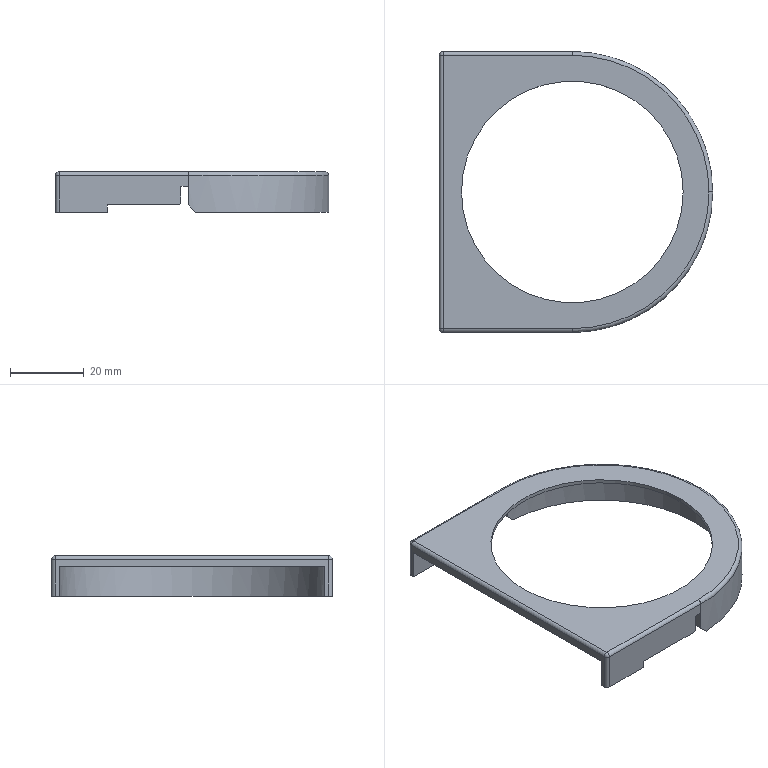Part | SolidWorks | features ICE 8, Fillet 2, Chamfer 1, Stock 1, SurfCut 1 | 1 solid | 39 faces | box 74 x 76 x 11 mm | volume 5943 mm3 | plane 24 | cylinder 11 | torus 2 | sphere 2 | commonest cylinder face diameters 2 x7 60 x2 72 x1 76 x1
STEP:
#1=CARTESIAN_POINT('',(133.,0.,24.));
#2=VERTEX_POINT('',#1);
#3=CARTESIAN_POINT('',(95.,-38.,24.));
#4=VERTEX_POINT('',#3);
#5=CARTESIAN_POINT('',(95.,0.,24.));
#6=DIRECTION('',(0.,0.,-1.));
#7=DIRECTION('',(1.,0.,0.));
#8=AXIS2_PLACEMENT_3D('',#5,#6,#7);
#9=CIRCLE('',#8,38.);
#10=EDGE_CURVE('',#2,#4,#9,.T.);
#11=ORIENTED_EDGE('',*,*,#10,.F.);
#12=CARTESIAN_POINT('',(132.,0.,25.));
#13=VERTEX_POINT('',#12);
#14=CARTESIAN_POINT('',(132.,0.,24.));
#15=DIRECTION('',(0.,-1.,0.));
#16=DIRECTION('',(0.,0.,-1.));
#17=AXIS2_PLACEMENT_3D('',#14,#15,#16);
#18=CIRCLE('',#17,1.);
#19=EDGE_CURVE('',#2,#13,#18,.T.);
#20=ORIENTED_EDGE('',*,*,#19,.T.);
#21=CARTESIAN_POINT('',(95.,-37.,25.));
#22=VERTEX_POINT('',#21);
#23=CARTESIAN_POINT('',(95.,0.,25.));
#24=DIRECTION('',(0.,0.,1.));
#25=DIRECTION('',(1.,0.,0.));
#26=AXIS2_PLACEMENT_3D('',#23,#24,#25);
#27=CIRCLE('',#26,37.);
#28=EDGE_CURVE('',#22,#13,#27,.T.);
#29=ORIENTED_EDGE('',*,*,#28,.F.);
#30=CARTESIAN_POINT('',(95.,-37.,24.));
#31=DIRECTION('',(1.,0.,0.));
#32=DIRECTION('',(0.,0.,-1.));
#33=AXIS2_PLACEMENT_3D('',#30,#31,#32);
#34=CIRCLE('',#33,1.);
#35=EDGE_CURVE('',#22,#4,#34,.T.);
#36=ORIENTED_EDGE('',*,*,#35,.T.);
#37=EDGE_LOOP('',(#11,#20,#29,#36));
#38=FACE_OUTER_BOUND('',#37,.T.);
#39=CARTESIAN_POINT('',(95.,0.,24.));
#40=DIRECTION('',(0.,0.,1.));
#41=DIRECTION('',(1.,0.,0.));
#42=AXIS2_PLACEMENT_3D('',#39,#40,#41);
#43=TOROIDAL_SURFACE('',#42,37.,1.);
#44=ADVANCED_FACE('',(#38),#43,.T.);
#45=CARTESIAN_POINT('',(65.,0.,24.));
#46=VERTEX_POINT('',#45);
#47=CARTESIAN_POINT('',(125.,0.,24.));
#48=VERTEX_POINT('',#47);
#49=CARTESIAN_POINT('',(95.,0.,24.));
#50=DIRECTION('',(0.,0.,1.));
#51=DIRECTION('',(1.,0.,0.));
#52=AXIS2_PLACEMENT_3D('',#49,#50,#51);
#53=CIRCLE('',#52,30.);
#54=EDGE_CURVE('',#46,#48,#53,.T.);
#55=ORIENTED_EDGE('',*,*,#54,.F.);
#56=CARTESIAN_POINT('',(65.,0.,25.));
#57=VERTEX_POINT('',#56);
#58=CARTESIAN_POINT('',(65.,0.,18.));
#59=DIRECTION('',(0.,0.,1.));
#60=VECTOR('',#59,1000.);
#61=LINE('',#58,#60);
#62=EDGE_CURVE('',#46,#57,#61,.T.);
#63=ORIENTED_EDGE('',*,*,#62,.T.);
#64=CARTESIAN_POINT('',(125.,0.,25.));
#65=VERTEX_POINT('',#64);
#66=CARTESIAN_POINT('',(95.,0.,25.));
#67=DIRECTION('',(0.,0.,1.));
#68=DIRECTION('',(1.,0.,0.));
#69=AXIS2_PLACEMENT_3D('',#66,#67,#68);
#70=CIRCLE('',#69,30.);
#71=EDGE_CURVE('',#57,#65,#70,.T.);
#72=ORIENTED_EDGE('',*,*,#71,.T.);
#73=CARTESIAN_POINT('',(125.,0.,18.));
#74=DIRECTION('',(0.,0.,1.));
#75=VECTOR('',#74,1000.);
#76=LINE('',#73,#75);
#77=EDGE_CURVE('',#48,#65,#76,.T.);
#78=ORIENTED_EDGE('',*,*,#77,.F.);
#79=EDGE_LOOP('',(#55,#63,#72,#78));
#80=FACE_OUTER_BOUND('',#79,.T.);
#81=CARTESIAN_POINT('',(95.,0.,18.));
#82=DIRECTION('',(0.,0.,1.));
#83=DIRECTION('',(1.,0.,0.));
#84=AXIS2_PLACEMENT_3D('',#81,#82,#83);
#85=CYLINDRICAL_SURFACE('',#84,30.);
#86=ADVANCED_FACE('',(#80),#85,.F.);
#87=CARTESIAN_POINT('',(95.,0.,24.));
#88=DIRECTION('',(0.,0.,1.));
#89=DIRECTION('',(1.,0.,0.));
#90=AXIS2_PLACEMENT_3D('',#87,#88,#89);
#91=CIRCLE('',#90,30.);
#92=EDGE_CURVE('',#48,#46,#91,.T.);
#93=ORIENTED_EDGE('',*,*,#92,.T.);
#94=ORIENTED_EDGE('',*,*,#54,.T.);
#95=EDGE_LOOP('',(#93,#94));
#96=FACE_BOUND('',#95,.T.);
#97=CARTESIAN_POINT('',(61.,36.,24.));
#98=VERTEX_POINT('',#97);
#99=CARTESIAN_POINT('',(61.,-36.,24.));
#100=VERTEX_POINT('',#99);
#101=CARTESIAN_POINT('',(61.,-34.,24.));
#102=DIRECTION('',(0.,-1.,0.));
#103=VECTOR('',#102,1000.);
#104=LINE('',#101,#103);
#105=EDGE_CURVE('',#98,#100,#104,.T.);
#106=ORIENTED_EDGE('',*,*,#105,.F.);
#107=CARTESIAN_POINT('',(95.,36.,24.));
#108=VERTEX_POINT('',#107);
#109=CARTESIAN_POINT('',(61.,36.,24.));
#110=DIRECTION('',(1.,0.,0.));
#111=VECTOR('',#110,1000.);
#112=LINE('',#109,#111);
#113=EDGE_CURVE('',#98,#108,#112,.T.);
#114=ORIENTED_EDGE('',*,*,#113,.T.);
#115=CARTESIAN_POINT('',(95.,-36.,24.));
#116=VERTEX_POINT('',#115);
#117=CARTESIAN_POINT('',(95.,0.,24.));
#118=DIRECTION('',(0.,0.,-1.));
#119=DIRECTION('',(1.,0.,0.));
#120=AXIS2_PLACEMENT_3D('',#117,#118,#119);
#121=CIRCLE('',#120,36.);
#122=EDGE_CURVE('',#108,#116,#121,.T.);
#123=ORIENTED_EDGE('',*,*,#122,.T.);
#124=CARTESIAN_POINT('',(73.,-36.,24.));
#125=DIRECTION('',(-1.,0.,0.));
#126=VECTOR('',#125,1000.);
#127=LINE('',#124,#126);
#128=EDGE_CURVE('',#116,#100,#127,.T.);
#129=ORIENTED_EDGE('',*,*,#128,.T.);
#130=EDGE_LOOP('',(#106,#114,#123,#129));
#131=FACE_OUTER_BOUND('',#130,.T.);
#132=CARTESIAN_POINT('',(95.,0.,24.));
#133=DIRECTION('',(0.,0.,1.));
#134=DIRECTION('',(1.,0.,0.));
#135=AXIS2_PLACEMENT_3D('',#132,#133,#134);
#136=PLANE('',#135);
#137=ADVANCED_FACE('',(#96,#131),#136,.F.);
#138=CARTESIAN_POINT('',(59.,-37.,14.));
#139=VERTEX_POINT('',#138);
#140=CARTESIAN_POINT('',(59.,-36.,14.));
#141=VERTEX_POINT('',#140);
#142=CARTESIAN_POINT('',(59.,-49.18,14.));
#143=DIRECTION('',(0.,1.,0.));
#144=VECTOR('',#143,1000.);
#145=LINE('',#142,#144);
#146=EDGE_CURVE('',#139,#141,#145,.T.);
#147=ORIENTED_EDGE('',*,*,#146,.T.);
#148=CARTESIAN_POINT('',(73.,-36.,14.));
#149=VERTEX_POINT('',#148);
#150=CARTESIAN_POINT('',(73.,-36.,14.));
#151=DIRECTION('',(-1.,0.,0.));
#152=VECTOR('',#151,1000.);
#153=LINE('',#150,#152);
#154=EDGE_CURVE('',#149,#141,#153,.T.);
#155=ORIENTED_EDGE('',*,*,#154,.F.);
#156=CARTESIAN_POINT('',(73.,-38.,14.));
#157=VERTEX_POINT('',#156);
#158=CARTESIAN_POINT('',(73.,-44.,14.));
#159=DIRECTION('',(0.,1.,0.));
#160=VECTOR('',#159,1000.);
#161=LINE('',#158,#160);
#162=EDGE_CURVE('',#157,#149,#161,.T.);
#163=ORIENTED_EDGE('',*,*,#162,.F.);
#164=CARTESIAN_POINT('',(60.,-38.,14.));
#165=VERTEX_POINT('',#164);
#166=CARTESIAN_POINT('',(2.,-38.,14.));
#167=DIRECTION('',(1.,0.,0.));
#168=VECTOR('',#167,1000.);
#169=LINE('',#166,#168);
#170=EDGE_CURVE('',#165,#157,#169,.T.);
#171=ORIENTED_EDGE('',*,*,#170,.F.);
#172=CARTESIAN_POINT('',(60.,-37.,14.));
#173=DIRECTION('',(0.,0.,-1.));
#174=DIRECTION('',(1.,0.,0.));
#175=AXIS2_PLACEMENT_3D('',#172,#173,#174);
#176=CIRCLE('',#175,1.);
#177=EDGE_CURVE('',#165,#139,#176,.T.);
#178=ORIENTED_EDGE('',*,*,#177,.T.);
#179=EDGE_LOOP('',(#147,#155,#163,#171,#178));
#180=FACE_OUTER_BOUND('',#179,.T.);
#181=CARTESIAN_POINT('',(57.,-50.,14.));
#182=DIRECTION('',(0.,0.,1.));
#183=DIRECTION('',(1.,0.,0.));
#184=AXIS2_PLACEMENT_3D('',#181,#182,#183);
#185=PLANE('',#184);
#186=ADVANCED_FACE('',(#180),#185,.F.);
#187=CARTESIAN_POINT('',(73.,36.,14.));
#188=VERTEX_POINT('',#187);
#189=CARTESIAN_POINT('',(73.,38.,14.));
#190=VERTEX_POINT('',#189);
#191=CARTESIAN_POINT('',(73.,-44.,14.));
#192=DIRECTION('',(0.,1.,0.));
#193=VECTOR('',#192,1000.);
#194=LINE('',#191,#193);
#195=EDGE_CURVE('',#188,#190,#194,.T.);
#196=ORIENTED_EDGE('',*,*,#195,.F.);
#197=CARTESIAN_POINT('',(59.,36.,14.));
#198=VERTEX_POINT('',#197);
#199=CARTESIAN_POINT('',(61.,36.,14.));
#200=DIRECTION('',(1.,0.,0.));
#201=VECTOR('',#200,1000.);
#202=LINE('',#199,#201);
#203=EDGE_CURVE('',#198,#188,#202,.T.);
#204=ORIENTED_EDGE('',*,*,#203,.F.);
#205=CARTESIAN_POINT('',(59.,37.,14.));
#206=VERTEX_POINT('',#205);
#207=CARTESIAN_POINT('',(59.,-49.18,14.));
#208=DIRECTION('',(0.,1.,0.));
#209=VECTOR('',#208,1000.);
#210=LINE('',#207,#209);
#211=EDGE_CURVE('',#198,#206,#210,.T.);
#212=ORIENTED_EDGE('',*,*,#211,.T.);
#213=CARTESIAN_POINT('',(60.,38.,14.));
#214=VERTEX_POINT('',#213);
#215=CARTESIAN_POINT('',(60.,37.,14.));
#216=DIRECTION('',(0.,0.,-1.));
#217=DIRECTION('',(1.,0.,0.));
#218=AXIS2_PLACEMENT_3D('',#215,#216,#217);
#219=CIRCLE('',#218,1.);
#220=EDGE_CURVE('',#206,#214,#219,.T.);
#221=ORIENTED_EDGE('',*,*,#220,.T.);
#222=CARTESIAN_POINT('',(95.,38.,14.));
#223=DIRECTION('',(-1.,0.,0.));
#224=VECTOR('',#223,1000.);
#225=LINE('',#222,#224);
#226=EDGE_CURVE('',#190,#214,#225,.T.);
#227=ORIENTED_EDGE('',*,*,#226,.F.);
#228=EDGE_LOOP('',(#196,#204,#212,#221,#227));
#229=FACE_OUTER_BOUND('',#228,.T.);
#230=CARTESIAN_POINT('',(57.,-50.,14.));
#231=DIRECTION('',(0.,0.,1.));
#232=DIRECTION('',(1.,0.,0.));
#233=AXIS2_PLACEMENT_3D('',#230,#231,#232);
#234=PLANE('',#233);
#235=ADVANCED_FACE('',(#229),#234,.F.);
#236=CARTESIAN_POINT('',(61.,-36.,22.));
#237=VERTEX_POINT('',#236);
#238=CARTESIAN_POINT('',(61.,36.,22.));
#239=VERTEX_POINT('',#238);
#240=CARTESIAN_POINT('',(61.,-41.606,22.));
#241=DIRECTION('',(0.,1.,0.));
#242=VECTOR('',#241,1000.);
#243=LINE('',#240,#242);
#244=EDGE_CURVE('',#237,#239,#243,.T.);
#245=ORIENTED_EDGE('',*,*,#244,.T.);
#246=CARTESIAN_POINT('',(61.,36.,22.));
#247=DIRECTION('',(0.,0.,-1.));
#248=VECTOR('',#247,1000.);
#249=LINE('',#246,#248);
#250=EDGE_CURVE('',#98,#239,#249,.T.);
#251=ORIENTED_EDGE('',*,*,#250,.F.);
#252=ORIENTED_EDGE('',*,*,#105,.T.);
#253=CARTESIAN_POINT('',(61.,-36.,22.));
#254=DIRECTION('',(0.,0.,1.));
#255=VECTOR('',#254,1000.);
#256=LINE('',#253,#255);
#257=EDGE_CURVE('',#237,#100,#256,.T.);
#258=ORIENTED_EDGE('',*,*,#257,.F.);
#259=EDGE_LOOP('',(#245,#251,#252,#258));
#260=FACE_OUTER_BOUND('',#259,.T.);
#261=CARTESIAN_POINT('',(61.,-41.606,22.));
#262=DIRECTION('',(1.,0.,0.));
#263=DIRECTION('',(0.,1.,0.));
#264=AXIS2_PLACEMENT_3D('',#261,#262,#263);
#265=PLANE('',#264);
#266=ADVANCED_FACE('',(#260),#265,.T.);
#267=CARTESIAN_POINT('',(97.,-37.947,14.));
#268=VERTEX_POINT('',#267);
#269=CARTESIAN_POINT('',(97.,37.947,14.));
#270=VERTEX_POINT('',#269);
#271=CARTESIAN_POINT('',(95.,0.,14.));
#272=DIRECTION('',(0.,0.,1.));
#273=DIRECTION('',(1.,0.,0.));
#274=AXIS2_PLACEMENT_3D('',#271,#272,#273);
#275=CIRCLE('',#274,38.);
#276=EDGE_CURVE('',#268,#270,#275,.T.);
#277=ORIENTED_EDGE('',*,*,#276,.F.);
#278=CARTESIAN_POINT('',(97.,-35.944,14.));
#279=VERTEX_POINT('',#278);
#280=CARTESIAN_POINT('',(97.,-50.,14.));
#281=DIRECTION('',(0.,1.,0.));
#282=VECTOR('',#281,1000.);
#283=LINE('',#280,#282);
#284=EDGE_CURVE('',#268,#279,#283,.T.);
#285=ORIENTED_EDGE('',*,*,#284,.T.);
#286=CARTESIAN_POINT('',(97.,35.944,14.));
#287=VERTEX_POINT('',#286);
#288=CARTESIAN_POINT('',(95.,0.,14.));
#289=DIRECTION('',(0.,0.,-1.));
#290=DIRECTION('',(-1.,0.,0.));
#291=AXIS2_PLACEMENT_3D('',#288,#289,#290);
#292=CIRCLE('',#291,36.);
#293=EDGE_CURVE('',#287,#279,#292,.T.);
#294=ORIENTED_EDGE('',*,*,#293,.F.);
#295=CARTESIAN_POINT('',(97.,-50.,14.));
#296=DIRECTION('',(0.,1.,0.));
#297=VECTOR('',#296,1000.);
#298=LINE('',#295,#297);
#299=EDGE_CURVE('',#287,#270,#298,.T.);
#300=ORIENTED_EDGE('',*,*,#299,.T.);
#301=EDGE_LOOP('',(#277,#285,#294,#300));
#302=FACE_OUTER_BOUND('',#301,.T.);
#303=CARTESIAN_POINT('',(57.,-50.,14.));
#304=DIRECTION('',(0.,0.,1.));
#305=DIRECTION('',(1.,0.,0.));
#306=AXIS2_PLACEMENT_3D('',#303,#304,#305);
#307=PLANE('',#306);
#308=ADVANCED_FACE('',(#302),#307,.F.);
#309=CARTESIAN_POINT('',(93.,38.,21.));
#310=VERTEX_POINT('',#309);
#311=CARTESIAN_POINT('',(93.,38.,17.));
#312=VERTEX_POINT('',#311);
#313=CARTESIAN_POINT('',(93.,38.,25.));
#314=DIRECTION('',(0.,0.,-1.));
#315=VECTOR('',#314,1000.);
#316=LINE('',#313,#315);
#317=EDGE_CURVE('',#310,#312,#316,.T.);
#318=ORIENTED_EDGE('',*,*,#317,.T.);
#319=CARTESIAN_POINT('',(92.,38.,16.));
#320=VERTEX_POINT('',#319);
#321=CARTESIAN_POINT('',(92.,38.,17.));
#322=DIRECTION('',(0.,1.,0.));
#323=DIRECTION('',(1.,0.,0.));
#324=AXIS2_PLACEMENT_3D('',#321,#322,#323);
#325=CIRCLE('',#324,1.);
#326=EDGE_CURVE('',#312,#320,#325,.T.);
#327=ORIENTED_EDGE('',*,*,#326,.T.);
#328=CARTESIAN_POINT('',(73.,38.,16.));
#329=VERTEX_POINT('',#328);
#330=CARTESIAN_POINT('',(95.,38.,16.));
#331=DIRECTION('',(-1.,0.,0.));
#332=VECTOR('',#331,1000.);
#333=LINE('',#330,#332);
#334=EDGE_CURVE('',#320,#329,#333,.T.);
#335=ORIENTED_EDGE('',*,*,#334,.T.);
#336=CARTESIAN_POINT('',(73.,38.,25.));
#337=DIRECTION('',(0.,0.,-1.));
#338=VECTOR('',#337,1000.);
#339=LINE('',#336,#338);
#340=EDGE_CURVE('',#329,#190,#339,.T.);
#341=ORIENTED_EDGE('',*,*,#340,.T.);
#342=ORIENTED_EDGE('',*,*,#226,.T.);
#343=CARTESIAN_POINT('',(60.,38.,24.));
#344=VERTEX_POINT('',#343);
#345=CARTESIAN_POINT('',(60.,38.,25.));
#346=DIRECTION('',(0.,0.,1.));
#347=VECTOR('',#346,1000.);
#348=LINE('',#345,#347);
#349=EDGE_CURVE('',#214,#344,#348,.T.);
#350=ORIENTED_EDGE('',*,*,#349,.T.);
#351=CARTESIAN_POINT('',(95.,38.,24.));
#352=VERTEX_POINT('',#351);
#353=CARTESIAN_POINT('',(95.,38.,24.));
#354=DIRECTION('',(1.,0.,0.));
#355=VECTOR('',#354,1000.);
#356=LINE('',#353,#355);
#357=EDGE_CURVE('',#344,#352,#356,.T.);
#358=ORIENTED_EDGE('',*,*,#357,.T.);
#359=CARTESIAN_POINT('',(95.,38.,21.));
#360=VERTEX_POINT('',#359);
#361=CARTESIAN_POINT('',(95.,38.,25.));
#362=DIRECTION('',(0.,0.,-1.));
#363=VECTOR('',#362,1000.);
#364=LINE('',#361,#363);
#365=EDGE_CURVE('',#352,#360,#364,.T.);
#366=ORIENTED_EDGE('',*,*,#365,.T.);
#367=CARTESIAN_POINT('',(95.,38.,21.));
#368=DIRECTION('',(-1.,0.,0.));
#369=VECTOR('',#368,1000.);
#370=LINE('',#367,#369);
#371=EDGE_CURVE('',#360,#310,#370,.T.);
#372=ORIENTED_EDGE('',*,*,#371,.T.);
#373=EDGE_LOOP('',(#318,#327,#335,#341,#342,#350,#358,#366,#372));
#374=FACE_OUTER_BOUND('',#373,.T.);
#375=CARTESIAN_POINT('',(95.,38.,25.));
#376=DIRECTION('',(0.,-1.,0.));
#377=DIRECTION('',(1.,0.,0.));
#378=AXIS2_PLACEMENT_3D('',#375,#376,#377);
#379=PLANE('',#378);
#380=ADVANCED_FACE('',(#374),#379,.F.);
#381=CARTESIAN_POINT('',(73.,-38.,16.));
#382=VERTEX_POINT('',#381);
#383=CARTESIAN_POINT('',(92.,-38.,16.));
#384=VERTEX_POINT('',#383);
#385=CARTESIAN_POINT('',(2.,-38.,16.));
#386=DIRECTION('',(1.,0.,0.));
#387=VECTOR('',#386,1000.);
#388=LINE('',#385,#387);
#389=EDGE_CURVE('',#382,#384,#388,.T.);
#390=ORIENTED_EDGE('',*,*,#389,.T.);
#391=CARTESIAN_POINT('',(93.,-38.,17.));
#392=VERTEX_POINT('',#391);
#393=CARTESIAN_POINT('',(92.,-38.,17.));
#394=DIRECTION('',(0.,-1.,0.));
#395=DIRECTION('',(-1.,0.,0.));
#396=AXIS2_PLACEMENT_3D('',#393,#394,#395);
#397=CIRCLE('',#396,1.);
#398=EDGE_CURVE('',#384,#392,#397,.T.);
#399=ORIENTED_EDGE('',*,*,#398,.T.);
#400=CARTESIAN_POINT('',(93.,-38.,21.));
#401=VERTEX_POINT('',#400);
#402=CARTESIAN_POINT('',(93.,-38.,25.));
#403=DIRECTION('',(0.,0.,1.));
#404=VECTOR('',#403,1000.);
#405=LINE('',#402,#404);
#406=EDGE_CURVE('',#392,#401,#405,.T.);
#407=ORIENTED_EDGE('',*,*,#406,.T.);
#408=CARTESIAN_POINT('',(95.,-38.,21.));
#409=VERTEX_POINT('',#408);
#410=CARTESIAN_POINT('',(2.,-38.,21.));
#411=DIRECTION('',(1.,0.,0.));
#412=VECTOR('',#411,1000.);
#413=LINE('',#410,#412);
#414=EDGE_CURVE('',#401,#409,#413,.T.);
#415=ORIENTED_EDGE('',*,*,#414,.T.);
#416=CARTESIAN_POINT('',(95.,-38.,25.));
#417=DIRECTION('',(0.,0.,-1.));
#418=VECTOR('',#417,1000.);
#419=LINE('',#416,#418);
#420=EDGE_CURVE('',#4,#409,#419,.T.);
#421=ORIENTED_EDGE('',*,*,#420,.F.);
#422=CARTESIAN_POINT('',(60.,-38.,24.));
#423=VERTEX_POINT('',#422);
#424=CARTESIAN_POINT('',(59.,-38.,24.));
#425=DIRECTION('',(-1.,0.,0.));
#426=VECTOR('',#425,1000.);
#427=LINE('',#424,#426);
#428=EDGE_CURVE('',#4,#423,#427,.T.);
#429=ORIENTED_EDGE('',*,*,#428,.T.);
#430=CARTESIAN_POINT('',(60.,-38.,25.));
#431=DIRECTION('',(0.,0.,-1.));
#432=VECTOR('',#431,1000.);
#433=LINE('',#430,#432);
#434=EDGE_CURVE('',#423,#165,#433,.T.);
#435=ORIENTED_EDGE('',*,*,#434,.T.);
#436=ORIENTED_EDGE('',*,*,#170,.T.);
#437=CARTESIAN_POINT('',(73.,-38.,25.));
#438=DIRECTION('',(0.,0.,1.));
#439=VECTOR('',#438,1000.);
#440=LINE('',#437,#439);
#441=EDGE_CURVE('',#157,#382,#440,.T.);
#442=ORIENTED_EDGE('',*,*,#441,.T.);
#443=EDGE_LOOP('',(#390,#399,#407,#415,#421,#429,#435,#436,#442));
#444=FACE_OUTER_BOUND('',#443,.T.);
#445=CARTESIAN_POINT('',(2.,-38.,25.));
#446=DIRECTION('',(0.,1.,0.));
#447=DIRECTION('',(-1.,0.,0.));
#448=AXIS2_PLACEMENT_3D('',#445,#446,#447);
#449=PLANE('',#448);
#450=ADVANCED_FACE('',(#444),#449,.F.);
#451=ORIENTED_EDGE('',*,*,#28,.T.);
#452=CARTESIAN_POINT('',(95.,37.,25.));
#453=VERTEX_POINT('',#452);
#454=CARTESIAN_POINT('',(95.,0.,25.));
#455=DIRECTION('',(0.,0.,1.));
#456=DIRECTION('',(1.,0.,0.));
#457=AXIS2_PLACEMENT_3D('',#454,#455,#456);
#458=CIRCLE('',#457,37.);
#459=EDGE_CURVE('',#13,#453,#458,.T.);
#460=ORIENTED_EDGE('',*,*,#459,.T.);
#461=CARTESIAN_POINT('',(60.,37.,25.));
#462=VERTEX_POINT('',#461);
#463=CARTESIAN_POINT('',(59.,37.,25.));
#464=DIRECTION('',(-1.,0.,0.));
#465=VECTOR('',#464,1000.);
#466=LINE('',#463,#465);
#467=EDGE_CURVE('',#453,#462,#466,.T.);
#468=ORIENTED_EDGE('',*,*,#467,.T.);
#469=CARTESIAN_POINT('',(60.,-37.,25.));
#470=VERTEX_POINT('',#469);
#471=CARTESIAN_POINT('',(60.,-38.,25.));
#472=DIRECTION('',(0.,-1.,0.));
#473=VECTOR('',#472,1000.);
#474=LINE('',#471,#473);
#475=EDGE_CURVE('',#462,#470,#474,.T.);
#476=ORIENTED_EDGE('',*,*,#475,.T.);
#477=CARTESIAN_POINT('',(95.,-37.,25.));
#478=DIRECTION('',(1.,0.,0.));
#479=VECTOR('',#478,1000.);
#480=LINE('',#477,#479);
#481=EDGE_CURVE('',#470,#22,#480,.T.);
#482=ORIENTED_EDGE('',*,*,#481,.T.);
#483=EDGE_LOOP('',(#451,#460,#468,#476,#482));
#484=FACE_OUTER_BOUND('',#483,.T.);
#485=CARTESIAN_POINT('',(95.,0.,25.));
#486=DIRECTION('',(0.,0.,1.));
#487=DIRECTION('',(1.,0.,0.));
#488=AXIS2_PLACEMENT_3D('',#485,#486,#487);
#489=CIRCLE('',#488,30.);
#490=EDGE_CURVE('',#65,#57,#489,.T.);
#491=ORIENTED_EDGE('',*,*,#490,.F.);
#492=ORIENTED_EDGE('',*,*,#71,.F.);
#493=EDGE_LOOP('',(#491,#492));
#494=FACE_BOUND('',#493,.T.);
#495=CARTESIAN_POINT('',(95.,0.,25.));
#496=DIRECTION('',(0.,0.,1.));
#497=DIRECTION('',(1.,0.,0.));
#498=AXIS2_PLACEMENT_3D('',#495,#496,#497);
#499=PLANE('',#498);
#500=ADVANCED_FACE('',(#484,#494),#499,.T.);
#501=CARTESIAN_POINT('',(95.,-38.,16.));
#502=VERTEX_POINT('',#501);
#503=CARTESIAN_POINT('',(95.,-38.,25.));
#504=DIRECTION('',(0.,0.,-1.));
#505=VECTOR('',#504,1000.);
#506=LINE('',#503,#505);
#507=EDGE_CURVE('',#409,#502,#506,.T.);
#508=ORIENTED_EDGE('',*,*,#507,.T.);
#509=CARTESIAN_POINT('',(95.,-38.,16.));
#510=CARTESIAN_POINT('',(95.667,-38.,15.333));
#511=CARTESIAN_POINT('',(96.334,-37.982,14.666));
#512=CARTESIAN_POINT('',(97.,-37.947,14.));
#513=(BOUNDED_CURVE()B_SPLINE_CURVE(3,(#509,#510,#511,#512),.UNSPECIFIED.,.F.,.F.)B_SPLINE_CURVE_WITH_KNOTS((4,4),(4.712,4.765),.UNSPECIFIED.)CURVE()GEOMETRIC_REPRESENTATION_ITEM()RATIONAL_B_SPLINE_CURVE((1.,0.9998,0.9998,1.))REPRESENTATION_ITEM(''));
#514=EDGE_CURVE('',#502,#268,#513,.T.);
#515=ORIENTED_EDGE('',*,*,#514,.T.);
#516=ORIENTED_EDGE('',*,*,#276,.T.);
#517=CARTESIAN_POINT('',(95.,38.,16.));
#518=VERTEX_POINT('',#517);
#519=CARTESIAN_POINT('',(97.,37.947,14.));
#520=CARTESIAN_POINT('',(96.334,37.982,14.666));
#521=CARTESIAN_POINT('',(95.667,38.,15.333));
#522=CARTESIAN_POINT('',(95.,38.,16.));
#523=(BOUNDED_CURVE()B_SPLINE_CURVE(3,(#519,#520,#521,#522),.UNSPECIFIED.,.F.,.F.)B_SPLINE_CURVE_WITH_KNOTS((4,4),(1.518,1.571),.UNSPECIFIED.)CURVE()GEOMETRIC_REPRESENTATION_ITEM()RATIONAL_B_SPLINE_CURVE((1.,0.9998,0.9998,1.))REPRESENTATION_ITEM(''));
#524=EDGE_CURVE('',#270,#518,#523,.T.);
#525=ORIENTED_EDGE('',*,*,#524,.T.);
#526=CARTESIAN_POINT('',(95.,38.,25.));
#527=DIRECTION('',(0.,0.,-1.));
#528=VECTOR('',#527,1000.);
#529=LINE('',#526,#528);
#530=EDGE_CURVE('',#360,#518,#529,.T.);
#531=ORIENTED_EDGE('',*,*,#530,.F.);
#532=ORIENTED_EDGE('',*,*,#365,.F.);
#533=CARTESIAN_POINT('',(95.,0.,24.));
#534=DIRECTION('',(0.,0.,-1.));
#535=DIRECTION('',(1.,0.,0.));
#536=AXIS2_PLACEMENT_3D('',#533,#534,#535);
#537=CIRCLE('',#536,38.);
#538=EDGE_CURVE('',#352,#2,#537,.T.);
#539=ORIENTED_EDGE('',*,*,#538,.T.);
#540=ORIENTED_EDGE('',*,*,#10,.T.);
#541=ORIENTED_EDGE('',*,*,#420,.T.);
#542=EDGE_LOOP('',(#508,#515,#516,#525,#531,#532,#539,#540,#541));
#543=FACE_OUTER_BOUND('',#542,.T.);
#544=CARTESIAN_POINT('',(95.,0.,25.));
#545=DIRECTION('',(0.,0.,-1.));
#546=DIRECTION('',(-1.,0.,0.));
#547=AXIS2_PLACEMENT_3D('',#544,#545,#546);
#548=CYLINDRICAL_SURFACE('',#547,38.);
#549=ADVANCED_FACE('',(#543),#548,.T.);
#550=ORIENTED_EDGE('',*,*,#211,.F.);
#551=CARTESIAN_POINT('',(59.,36.,22.));
#552=VERTEX_POINT('',#551);
#553=CARTESIAN_POINT('',(59.,36.,125.823));
#554=DIRECTION('',(0.,0.,-1.));
#555=VECTOR('',#554,1000.);
#556=LINE('',#553,#555);
#557=EDGE_CURVE('',#552,#198,#556,.T.);
#558=ORIENTED_EDGE('',*,*,#557,.F.);
#559=CARTESIAN_POINT('',(59.,-36.,22.));
#560=VERTEX_POINT('',#559);
#561=CARTESIAN_POINT('',(59.,-41.606,22.));
#562=DIRECTION('',(0.,1.,0.));
#563=VECTOR('',#562,1000.);
#564=LINE('',#561,#563);
#565=EDGE_CURVE('',#560,#552,#564,.T.);
#566=ORIENTED_EDGE('',*,*,#565,.F.);
#567=CARTESIAN_POINT('',(59.,-36.,125.823));
#568=DIRECTION('',(0.,0.,-1.));
#569=VECTOR('',#568,1000.);
#570=LINE('',#567,#569);
#571=EDGE_CURVE('',#560,#141,#570,.T.);
#572=ORIENTED_EDGE('',*,*,#571,.T.);
#573=ORIENTED_EDGE('',*,*,#146,.F.);
#574=CARTESIAN_POINT('',(59.,-37.,24.));
#575=VERTEX_POINT('',#574);
#576=CARTESIAN_POINT('',(59.,-37.,22.));
#577=DIRECTION('',(0.,0.,1.));
#578=VECTOR('',#577,1000.);
#579=LINE('',#576,#578);
#580=EDGE_CURVE('',#139,#575,#579,.T.);
#581=ORIENTED_EDGE('',*,*,#580,.T.);
#582=CARTESIAN_POINT('',(59.,37.,24.));
#583=VERTEX_POINT('',#582);
#584=CARTESIAN_POINT('',(59.,38.,24.));
#585=DIRECTION('',(0.,1.,0.));
#586=VECTOR('',#585,1000.);
#587=LINE('',#584,#586);
#588=EDGE_CURVE('',#575,#583,#587,.T.);
#589=ORIENTED_EDGE('',*,*,#588,.T.);
#590=CARTESIAN_POINT('',(59.,37.,22.));
#591=DIRECTION('',(0.,0.,-1.));
#592=VECTOR('',#591,1000.);
#593=LINE('',#590,#592);
#594=EDGE_CURVE('',#583,#206,#593,.T.);
#595=ORIENTED_EDGE('',*,*,#594,.T.);
#596=EDGE_LOOP('',(#550,#558,#566,#572,#573,#581,#589,#595));
#597=FACE_OUTER_BOUND('',#596,.T.);
#598=CARTESIAN_POINT('',(59.,-46.,22.));
#599=DIRECTION('',(1.,0.,0.));
#600=DIRECTION('',(0.,0.,-1.));
#601=AXIS2_PLACEMENT_3D('',#598,#599,#600);
#602=PLANE('',#601);
#603=ADVANCED_FACE('',(#597),#602,.F.);
#604=ORIENTED_EDGE('',*,*,#565,.T.);
#605=CARTESIAN_POINT('',(61.,36.,22.));
#606=DIRECTION('',(-1.,0.,0.));
#607=VECTOR('',#606,1000.);
#608=LINE('',#605,#607);
#609=EDGE_CURVE('',#239,#552,#608,.T.);
#610=ORIENTED_EDGE('',*,*,#609,.F.);
#611=ORIENTED_EDGE('',*,*,#244,.F.);
#612=CARTESIAN_POINT('',(61.,-36.,22.));
#613=DIRECTION('',(-1.,0.,0.));
#614=VECTOR('',#613,1000.);
#615=LINE('',#612,#614);
#616=EDGE_CURVE('',#237,#560,#615,.T.);
#617=ORIENTED_EDGE('',*,*,#616,.T.);
#618=EDGE_LOOP('',(#604,#610,#611,#617));
#619=FACE_OUTER_BOUND('',#618,.T.);
#620=CARTESIAN_POINT('',(59.,-41.606,22.));
#621=DIRECTION('',(0.,0.,-1.));
#622=DIRECTION('',(-1.,0.,0.));
#623=AXIS2_PLACEMENT_3D('',#620,#621,#622);
#624=PLANE('',#623);
#625=ADVANCED_FACE('',(#619),#624,.T.);
#626=ORIENTED_EDGE('',*,*,#62,.F.);
#627=ORIENTED_EDGE('',*,*,#92,.F.);
#628=ORIENTED_EDGE('',*,*,#77,.T.);
#629=ORIENTED_EDGE('',*,*,#490,.T.);
#630=EDGE_LOOP('',(#626,#627,#628,#629));
#631=FACE_OUTER_BOUND('',#630,.T.);
#632=CARTESIAN_POINT('',(95.,0.,18.));
#633=DIRECTION('',(0.,0.,1.));
#634=DIRECTION('',(1.,0.,0.));
#635=AXIS2_PLACEMENT_3D('',#632,#633,#634);
#636=CYLINDRICAL_SURFACE('',#635,30.);
#637=ADVANCED_FACE('',(#631),#636,.F.);
#638=CARTESIAN_POINT('',(60.,-37.,24.));
#639=DIRECTION('',(0.,0.,1.));
#640=DIRECTION('',(1.,0.,0.));
#641=AXIS2_PLACEMENT_3D('',#638,#639,#640);
#642=CIRCLE('',#641,1.);
#643=EDGE_CURVE('',#575,#423,#642,.T.);
#644=ORIENTED_EDGE('',*,*,#643,.F.);
#645=ORIENTED_EDGE('',*,*,#580,.F.);
#646=ORIENTED_EDGE('',*,*,#177,.F.);
#647=ORIENTED_EDGE('',*,*,#434,.F.);
#648=EDGE_LOOP('',(#644,#645,#646,#647));
#649=FACE_OUTER_BOUND('',#648,.T.);
#650=CARTESIAN_POINT('',(60.,-37.,25.));
#651=DIRECTION('',(0.,0.,-1.));
#652=DIRECTION('',(-1.,0.,0.));
#653=AXIS2_PLACEMENT_3D('',#650,#651,#652);
#654=CYLINDRICAL_SURFACE('',#653,1.);
#655=ADVANCED_FACE('',(#649),#654,.T.);
#656=CARTESIAN_POINT('',(60.,-37.,24.));
#657=DIRECTION('',(0.,1.,0.));
#658=DIRECTION('',(0.,0.,-1.));
#659=AXIS2_PLACEMENT_3D('',#656,#657,#658);
#660=CIRCLE('',#659,1.);
#661=EDGE_CURVE('',#575,#470,#660,.T.);
#662=ORIENTED_EDGE('',*,*,#661,.F.);
#663=ORIENTED_EDGE('',*,*,#643,.T.);
#664=CARTESIAN_POINT('',(60.,-37.,24.));
#665=DIRECTION('',(1.,0.,0.));
#666=DIRECTION('',(0.,0.,1.));
#667=AXIS2_PLACEMENT_3D('',#664,#665,#666);
#668=CIRCLE('',#667,1.);
#669=EDGE_CURVE('',#470,#423,#668,.T.);
#670=ORIENTED_EDGE('',*,*,#669,.F.);
#671=EDGE_LOOP('',(#662,#663,#670));
#672=FACE_OUTER_BOUND('',#671,.T.);
#673=CARTESIAN_POINT('',(60.,-37.,24.));
#674=DIRECTION('',(0.,1.,0.));
#675=DIRECTION('',(1.,0.,0.));
#676=AXIS2_PLACEMENT_3D('',#673,#674,#675);
#677=SPHERICAL_SURFACE('',#676,1.);
#678=ADVANCED_FACE('',(#672),#677,.T.);
#679=ORIENTED_EDGE('',*,*,#669,.T.);
#680=ORIENTED_EDGE('',*,*,#428,.F.);
#681=ORIENTED_EDGE('',*,*,#35,.F.);
#682=ORIENTED_EDGE('',*,*,#481,.F.);
#683=EDGE_LOOP('',(#679,#680,#681,#682));
#684=FACE_OUTER_BOUND('',#683,.T.);
#685=CARTESIAN_POINT('',(95.,-37.,24.));
#686=DIRECTION('',(-1.,0.,0.));
#687=DIRECTION('',(0.,-1.,0.));
#688=AXIS2_PLACEMENT_3D('',#685,#686,#687);
#689=CYLINDRICAL_SURFACE('',#688,1.);
#690=ADVANCED_FACE('',(#684),#689,.T.);
#691=ORIENTED_EDGE('',*,*,#661,.T.);
#692=ORIENTED_EDGE('',*,*,#475,.F.);
#693=CARTESIAN_POINT('',(60.,37.,24.));
#694=DIRECTION('',(0.,1.,0.));
#695=DIRECTION('',(0.,0.,1.));
#696=AXIS2_PLACEMENT_3D('',#693,#694,#695);
#697=CIRCLE('',#696,1.);
#698=EDGE_CURVE('',#583,#462,#697,.T.);
#699=ORIENTED_EDGE('',*,*,#698,.F.);
#700=ORIENTED_EDGE('',*,*,#588,.F.);
#701=EDGE_LOOP('',(#691,#692,#699,#700));
#702=FACE_OUTER_BOUND('',#701,.T.);
#703=CARTESIAN_POINT('',(60.,-46.,24.));
#704=DIRECTION('',(0.,-1.,0.));
#705=DIRECTION('',(0.,0.,-1.));
#706=AXIS2_PLACEMENT_3D('',#703,#704,#705);
#707=CYLINDRICAL_SURFACE('',#706,1.);
#708=ADVANCED_FACE('',(#702),#707,.T.);
#709=ORIENTED_EDGE('',*,*,#220,.F.);
#710=ORIENTED_EDGE('',*,*,#594,.F.);
#711=CARTESIAN_POINT('',(60.,37.,24.));
#712=DIRECTION('',(0.,0.,1.));
#713=DIRECTION('',(1.,0.,0.));
#714=AXIS2_PLACEMENT_3D('',#711,#712,#713);
#715=CIRCLE('',#714,1.);
#716=EDGE_CURVE('',#344,#583,#715,.T.);
#717=ORIENTED_EDGE('',*,*,#716,.F.);
#718=ORIENTED_EDGE('',*,*,#349,.F.);
#719=EDGE_LOOP('',(#709,#710,#717,#718));
#720=FACE_OUTER_BOUND('',#719,.T.);
#721=CARTESIAN_POINT('',(60.,37.,25.));
#722=DIRECTION('',(0.,0.,1.));
#723=DIRECTION('',(1.,0.,0.));
#724=AXIS2_PLACEMENT_3D('',#721,#722,#723);
#725=CYLINDRICAL_SURFACE('',#724,1.);
#726=ADVANCED_FACE('',(#720),#725,.T.);
#727=ORIENTED_EDGE('',*,*,#19,.F.);
#728=ORIENTED_EDGE('',*,*,#538,.F.);
#729=CARTESIAN_POINT('',(95.,37.,24.));
#730=DIRECTION('',(-1.,0.,0.));
#731=DIRECTION('',(0.,0.,1.));
#732=AXIS2_PLACEMENT_3D('',#729,#730,#731);
#733=CIRCLE('',#732,1.);
#734=EDGE_CURVE('',#453,#352,#733,.T.);
#735=ORIENTED_EDGE('',*,*,#734,.F.);
#736=ORIENTED_EDGE('',*,*,#459,.F.);
#737=EDGE_LOOP('',(#727,#728,#735,#736));
#738=FACE_OUTER_BOUND('',#737,.T.);
#739=CARTESIAN_POINT('',(95.,0.,24.));
#740=DIRECTION('',(0.,0.,1.));
#741=DIRECTION('',(1.,0.,0.));
#742=AXIS2_PLACEMENT_3D('',#739,#740,#741);
#743=TOROIDAL_SURFACE('',#742,37.,1.);
#744=ADVANCED_FACE('',(#738),#743,.T.);
#745=ORIENTED_EDGE('',*,*,#716,.T.);
#746=ORIENTED_EDGE('',*,*,#698,.T.);
#747=CARTESIAN_POINT('',(60.,37.,24.));
#748=DIRECTION('',(1.,0.,0.));
#749=DIRECTION('',(0.,0.,1.));
#750=AXIS2_PLACEMENT_3D('',#747,#748,#749);
#751=CIRCLE('',#750,1.);
#752=EDGE_CURVE('',#344,#462,#751,.T.);
#753=ORIENTED_EDGE('',*,*,#752,.F.);
#754=EDGE_LOOP('',(#745,#746,#753));
#755=FACE_OUTER_BOUND('',#754,.T.);
#756=CARTESIAN_POINT('',(60.,37.,24.));
#757=DIRECTION('',(0.,1.,0.));
#758=DIRECTION('',(1.,0.,0.));
#759=AXIS2_PLACEMENT_3D('',#756,#757,#758);
#760=SPHERICAL_SURFACE('',#759,1.);
#761=ADVANCED_FACE('',(#755),#760,.T.);
#762=ORIENTED_EDGE('',*,*,#734,.T.);
#763=ORIENTED_EDGE('',*,*,#357,.F.);
#764=ORIENTED_EDGE('',*,*,#752,.T.);
#765=ORIENTED_EDGE('',*,*,#467,.F.);
#766=EDGE_LOOP('',(#762,#763,#764,#765));
#767=FACE_OUTER_BOUND('',#766,.T.);
#768=CARTESIAN_POINT('',(95.,37.,24.));
#769=DIRECTION('',(1.,0.,0.));
#770=DIRECTION('',(0.,1.,0.));
#771=AXIS2_PLACEMENT_3D('',#768,#769,#770);
#772=CYLINDRICAL_SURFACE('',#771,1.);
#773=ADVANCED_FACE('',(#767),#772,.T.);
#774=ORIENTED_EDGE('',*,*,#530,.T.);
#775=CARTESIAN_POINT('',(95.,36.,16.));
#776=VERTEX_POINT('',#775);
#777=CARTESIAN_POINT('',(95.,-38.5,16.));
#778=DIRECTION('',(0.,-1.,0.));
#779=VECTOR('',#778,1000.);
#780=LINE('',#777,#779);
#781=EDGE_CURVE('',#518,#776,#780,.T.);
#782=ORIENTED_EDGE('',*,*,#781,.T.);
#783=CARTESIAN_POINT('',(95.,36.,21.));
#784=VERTEX_POINT('',#783);
#785=CARTESIAN_POINT('',(95.,36.,125.823));
#786=DIRECTION('',(0.,0.,-1.));
#787=VECTOR('',#786,1000.);
#788=LINE('',#785,#787);
#789=EDGE_CURVE('',#784,#776,#788,.T.);
#790=ORIENTED_EDGE('',*,*,#789,.F.);
#791=CARTESIAN_POINT('',(95.,-38.5,21.));
#792=DIRECTION('',(0.,1.,0.));
#793=VECTOR('',#792,1000.);
#794=LINE('',#791,#793);
#795=EDGE_CURVE('',#784,#360,#794,.T.);
#796=ORIENTED_EDGE('',*,*,#795,.T.);
#797=EDGE_LOOP('',(#774,#782,#790,#796));
#798=FACE_OUTER_BOUND('',#797,.T.);
#799=CARTESIAN_POINT('',(95.,-38.5,21.));
#800=DIRECTION('',(1.,0.,0.));
#801=DIRECTION('',(0.,0.,-1.));
#802=AXIS2_PLACEMENT_3D('',#799,#800,#801);
#803=PLANE('',#802);
#804=ADVANCED_FACE('',(#798),#803,.F.);
#805=ORIENTED_EDGE('',*,*,#795,.F.);
#806=CARTESIAN_POINT('',(93.,36.,21.));
#807=VERTEX_POINT('',#806);
#808=CARTESIAN_POINT('',(93.,36.,21.));
#809=DIRECTION('',(-1.,0.,0.));
#810=VECTOR('',#809,1000.);
#811=LINE('',#808,#810);
#812=EDGE_CURVE('',#784,#807,#811,.T.);
#813=ORIENTED_EDGE('',*,*,#812,.T.);
#814=CARTESIAN_POINT('',(93.,-38.5,21.));
#815=DIRECTION('',(0.,1.,0.));
#816=VECTOR('',#815,1000.);
#817=LINE('',#814,#816);
#818=EDGE_CURVE('',#807,#310,#817,.T.);
#819=ORIENTED_EDGE('',*,*,#818,.T.);
#820=ORIENTED_EDGE('',*,*,#371,.F.);
#821=EDGE_LOOP('',(#805,#813,#819,#820));
#822=FACE_OUTER_BOUND('',#821,.T.);
#823=CARTESIAN_POINT('',(93.,-38.5,21.));
#824=DIRECTION('',(0.,0.,1.));
#825=DIRECTION('',(1.,0.,0.));
#826=AXIS2_PLACEMENT_3D('',#823,#824,#825);
#827=PLANE('',#826);
#828=ADVANCED_FACE('',(#822),#827,.F.);
#829=CARTESIAN_POINT('',(93.,36.,17.));
#830=VERTEX_POINT('',#829);
#831=CARTESIAN_POINT('',(93.,36.,21.));
#832=DIRECTION('',(0.,0.,-1.));
#833=VECTOR('',#832,1000.);
#834=LINE('',#831,#833);
#835=EDGE_CURVE('',#807,#830,#834,.T.);
#836=ORIENTED_EDGE('',*,*,#835,.T.);
#837=CARTESIAN_POINT('',(93.,-38.5,17.));
#838=DIRECTION('',(0.,1.,0.));
#839=VECTOR('',#838,1000.);
#840=LINE('',#837,#839);
#841=EDGE_CURVE('',#830,#312,#840,.T.);
#842=ORIENTED_EDGE('',*,*,#841,.T.);
#843=ORIENTED_EDGE('',*,*,#317,.F.);
#844=ORIENTED_EDGE('',*,*,#818,.F.);
#845=EDGE_LOOP('',(#836,#842,#843,#844));
#846=FACE_OUTER_BOUND('',#845,.T.);
#847=CARTESIAN_POINT('',(93.,-38.5,21.));
#848=DIRECTION('',(-1.,0.,0.));
#849=DIRECTION('',(0.,0.,1.));
#850=AXIS2_PLACEMENT_3D('',#847,#848,#849);
#851=PLANE('',#850);
#852=ADVANCED_FACE('',(#846),#851,.F.);
#853=ORIENTED_EDGE('',*,*,#406,.F.);
#854=CARTESIAN_POINT('',(93.,-36.,17.));
#855=VERTEX_POINT('',#854);
#856=CARTESIAN_POINT('',(93.,-38.5,17.));
#857=DIRECTION('',(0.,1.,0.));
#858=VECTOR('',#857,1000.);
#859=LINE('',#856,#858);
#860=EDGE_CURVE('',#392,#855,#859,.T.);
#861=ORIENTED_EDGE('',*,*,#860,.T.);
#862=CARTESIAN_POINT('',(93.,-36.,21.));
#863=VERTEX_POINT('',#862);
#864=CARTESIAN_POINT('',(93.,-36.,21.));
#865=DIRECTION('',(0.,0.,1.));
#866=VECTOR('',#865,1000.);
#867=LINE('',#864,#866);
#868=EDGE_CURVE('',#855,#863,#867,.T.);
#869=ORIENTED_EDGE('',*,*,#868,.T.);
#870=CARTESIAN_POINT('',(93.,-38.5,21.));
#871=DIRECTION('',(0.,1.,0.));
#872=VECTOR('',#871,1000.);
#873=LINE('',#870,#872);
#874=EDGE_CURVE('',#401,#863,#873,.T.);
#875=ORIENTED_EDGE('',*,*,#874,.F.);
#876=EDGE_LOOP('',(#853,#861,#869,#875));
#877=FACE_OUTER_BOUND('',#876,.T.);
#878=CARTESIAN_POINT('',(93.,-38.5,21.));
#879=DIRECTION('',(-1.,0.,0.));
#880=DIRECTION('',(0.,0.,1.));
#881=AXIS2_PLACEMENT_3D('',#878,#879,#880);
#882=PLANE('',#881);
#883=ADVANCED_FACE('',(#877),#882,.F.);
#884=CARTESIAN_POINT('',(95.,-36.,21.));
#885=VERTEX_POINT('',#884);
#886=CARTESIAN_POINT('',(95.,-36.,16.));
#887=VERTEX_POINT('',#886);
#888=CARTESIAN_POINT('',(95.,-36.,125.823));
#889=DIRECTION('',(0.,0.,-1.));
#890=VECTOR('',#889,1000.);
#891=LINE('',#888,#890);
#892=EDGE_CURVE('',#885,#887,#891,.T.);
#893=ORIENTED_EDGE('',*,*,#892,.T.);
#894=CARTESIAN_POINT('',(95.,-38.5,16.));
#895=DIRECTION('',(0.,-1.,0.));
#896=VECTOR('',#895,1000.);
#897=LINE('',#894,#896);
#898=EDGE_CURVE('',#887,#502,#897,.T.);
#899=ORIENTED_EDGE('',*,*,#898,.T.);
#900=ORIENTED_EDGE('',*,*,#507,.F.);
#901=CARTESIAN_POINT('',(95.,-38.5,21.));
#902=DIRECTION('',(0.,1.,0.));
#903=VECTOR('',#902,1000.);
#904=LINE('',#901,#903);
#905=EDGE_CURVE('',#409,#885,#904,.T.);
#906=ORIENTED_EDGE('',*,*,#905,.T.);
#907=EDGE_LOOP('',(#893,#899,#900,#906));
#908=FACE_OUTER_BOUND('',#907,.T.);
#909=CARTESIAN_POINT('',(95.,-38.5,21.));
#910=DIRECTION('',(1.,0.,0.));
#911=DIRECTION('',(0.,0.,-1.));
#912=AXIS2_PLACEMENT_3D('',#909,#910,#911);
#913=PLANE('',#912);
#914=ADVANCED_FACE('',(#908),#913,.F.);
#915=ORIENTED_EDGE('',*,*,#874,.T.);
#916=CARTESIAN_POINT('',(93.,-36.,21.));
#917=DIRECTION('',(1.,0.,0.));
#918=VECTOR('',#917,1000.);
#919=LINE('',#916,#918);
#920=EDGE_CURVE('',#863,#885,#919,.T.);
#921=ORIENTED_EDGE('',*,*,#920,.T.);
#922=ORIENTED_EDGE('',*,*,#905,.F.);
#923=ORIENTED_EDGE('',*,*,#414,.F.);
#924=EDGE_LOOP('',(#915,#921,#922,#923));
#925=FACE_OUTER_BOUND('',#924,.T.);
#926=CARTESIAN_POINT('',(93.,-38.5,21.));
#927=DIRECTION('',(0.,0.,1.));
#928=DIRECTION('',(1.,0.,0.));
#929=AXIS2_PLACEMENT_3D('',#926,#927,#928);
#930=PLANE('',#929);
#931=ADVANCED_FACE('',(#925),#930,.F.);
#932=CARTESIAN_POINT('',(73.,-36.,16.));
#933=VERTEX_POINT('',#932);
#934=CARTESIAN_POINT('',(92.,-36.,16.));
#935=VERTEX_POINT('',#934);
#936=CARTESIAN_POINT('',(93.,-36.,16.));
#937=DIRECTION('',(1.,0.,0.));
#938=VECTOR('',#937,1000.);
#939=LINE('',#936,#938);
#940=EDGE_CURVE('',#933,#935,#939,.T.);
#941=ORIENTED_EDGE('',*,*,#940,.T.);
#942=CARTESIAN_POINT('',(92.,-44.,16.));
#943=DIRECTION('',(0.,-1.,0.));
#944=VECTOR('',#943,1000.);
#945=LINE('',#942,#944);
#946=EDGE_CURVE('',#935,#384,#945,.T.);
#947=ORIENTED_EDGE('',*,*,#946,.T.);
#948=ORIENTED_EDGE('',*,*,#389,.F.);
#949=CARTESIAN_POINT('',(73.,-44.,16.));
#950=DIRECTION('',(0.,1.,0.));
#951=VECTOR('',#950,1000.);
#952=LINE('',#949,#951);
#953=EDGE_CURVE('',#382,#933,#952,.T.);
#954=ORIENTED_EDGE('',*,*,#953,.T.);
#955=EDGE_LOOP('',(#941,#947,#948,#954));
#956=FACE_OUTER_BOUND('',#955,.T.);
#957=CARTESIAN_POINT('',(93.,-44.,16.));
#958=DIRECTION('',(0.,0.,1.));
#959=DIRECTION('',(1.,0.,0.));
#960=AXIS2_PLACEMENT_3D('',#957,#958,#959);
#961=PLANE('',#960);
#962=ADVANCED_FACE('',(#956),#961,.F.);
#963=ORIENTED_EDGE('',*,*,#162,.T.);
#964=CARTESIAN_POINT('',(73.,-36.,14.));
#965=DIRECTION('',(0.,0.,1.));
#966=VECTOR('',#965,1000.);
#967=LINE('',#964,#966);
#968=EDGE_CURVE('',#149,#933,#967,.T.);
#969=ORIENTED_EDGE('',*,*,#968,.T.);
#970=ORIENTED_EDGE('',*,*,#953,.F.);
#971=ORIENTED_EDGE('',*,*,#441,.F.);
#972=EDGE_LOOP('',(#963,#969,#970,#971));
#973=FACE_OUTER_BOUND('',#972,.T.);
#974=CARTESIAN_POINT('',(73.,-44.,14.));
#975=DIRECTION('',(-1.,0.,0.));
#976=DIRECTION('',(0.,-1.,0.));
#977=AXIS2_PLACEMENT_3D('',#974,#975,#976);
#978=PLANE('',#977);
#979=ADVANCED_FACE('',(#973),#978,.F.);
#980=CARTESIAN_POINT('',(73.,36.,16.));
#981=VERTEX_POINT('',#980);
#982=CARTESIAN_POINT('',(73.,-44.,16.));
#983=DIRECTION('',(0.,1.,0.));
#984=VECTOR('',#983,1000.);
#985=LINE('',#982,#984);
#986=EDGE_CURVE('',#981,#329,#985,.T.);
#987=ORIENTED_EDGE('',*,*,#986,.F.);
#988=CARTESIAN_POINT('',(73.,36.,14.));
#989=DIRECTION('',(0.,0.,-1.));
#990=VECTOR('',#989,1000.);
#991=LINE('',#988,#990);
#992=EDGE_CURVE('',#981,#188,#991,.T.);
#993=ORIENTED_EDGE('',*,*,#992,.T.);
#994=ORIENTED_EDGE('',*,*,#195,.T.);
#995=ORIENTED_EDGE('',*,*,#340,.F.);
#996=EDGE_LOOP('',(#987,#993,#994,#995));
#997=FACE_OUTER_BOUND('',#996,.T.);
#998=CARTESIAN_POINT('',(73.,-44.,14.));
#999=DIRECTION('',(-1.,0.,0.));
#1000=DIRECTION('',(0.,-1.,0.));
#1001=AXIS2_PLACEMENT_3D('',#998,#999,#1000);
#1002=PLANE('',#1001);
#1003=ADVANCED_FACE('',(#997),#1002,.F.);
#1004=ORIENTED_EDGE('',*,*,#334,.F.);
#1005=CARTESIAN_POINT('',(92.,36.,16.));
#1006=VERTEX_POINT('',#1005);
#1007=CARTESIAN_POINT('',(92.,-44.,16.));
#1008=DIRECTION('',(0.,-1.,0.));
#1009=VECTOR('',#1008,1000.);
#1010=LINE('',#1007,#1009);
#1011=EDGE_CURVE('',#320,#1006,#1010,.T.);
#1012=ORIENTED_EDGE('',*,*,#1011,.T.);
#1013=CARTESIAN_POINT('',(93.,36.,16.));
#1014=DIRECTION('',(-1.,0.,0.));
#1015=VECTOR('',#1014,1000.);
#1016=LINE('',#1013,#1015);
#1017=EDGE_CURVE('',#1006,#981,#1016,.T.);
#1018=ORIENTED_EDGE('',*,*,#1017,.T.);
#1019=ORIENTED_EDGE('',*,*,#986,.T.);
#1020=EDGE_LOOP('',(#1004,#1012,#1018,#1019));
#1021=FACE_OUTER_BOUND('',#1020,.T.);
#1022=CARTESIAN_POINT('',(93.,-44.,16.));
#1023=DIRECTION('',(0.,0.,1.));
#1024=DIRECTION('',(1.,0.,0.));
#1025=AXIS2_PLACEMENT_3D('',#1022,#1023,#1024);
#1026=PLANE('',#1025);
#1027=ADVANCED_FACE('',(#1021),#1026,.F.);
#1028=ORIENTED_EDGE('',*,*,#868,.F.);
#1029=CARTESIAN_POINT('',(92.,-36.,17.));
#1030=DIRECTION('',(0.,1.,0.));
#1031=DIRECTION('',(1.,0.,0.));
#1032=AXIS2_PLACEMENT_3D('',#1029,#1030,#1031);
#1033=CIRCLE('',#1032,1.);
#1034=EDGE_CURVE('',#855,#935,#1033,.T.);
#1035=ORIENTED_EDGE('',*,*,#1034,.T.);
#1036=ORIENTED_EDGE('',*,*,#940,.F.);
#1037=ORIENTED_EDGE('',*,*,#968,.F.);
#1038=ORIENTED_EDGE('',*,*,#154,.T.);
#1039=ORIENTED_EDGE('',*,*,#571,.F.);
#1040=ORIENTED_EDGE('',*,*,#616,.F.);
#1041=ORIENTED_EDGE('',*,*,#257,.T.);
#1042=ORIENTED_EDGE('',*,*,#128,.F.);
#1043=CARTESIAN_POINT('',(95.,-36.,125.823));
#1044=DIRECTION('',(0.,0.,-1.));
#1045=VECTOR('',#1044,1000.);
#1046=LINE('',#1043,#1045);
#1047=EDGE_CURVE('',#116,#885,#1046,.T.);
#1048=ORIENTED_EDGE('',*,*,#1047,.T.);
#1049=ORIENTED_EDGE('',*,*,#920,.F.);
#1050=EDGE_LOOP('',(#1028,#1035,#1036,#1037,#1038,#1039,#1040,#1041,#1042,#1048,#1049));
#1051=FACE_OUTER_BOUND('',#1050,.T.);
#1052=CARTESIAN_POINT('',(73.,-36.,125.823));
#1053=DIRECTION('',(0.,-1.,0.));
#1054=DIRECTION('',(1.,0.,0.));
#1055=AXIS2_PLACEMENT_3D('',#1052,#1053,#1054);
#1056=PLANE('',#1055);
#1057=ADVANCED_FACE('',(#1051),#1056,.F.);
#1058=ORIENTED_EDGE('',*,*,#1017,.F.);
#1059=CARTESIAN_POINT('',(92.,36.,17.));
#1060=DIRECTION('',(0.,-1.,0.));
#1061=DIRECTION('',(-1.,0.,0.));
#1062=AXIS2_PLACEMENT_3D('',#1059,#1060,#1061);
#1063=CIRCLE('',#1062,1.);
#1064=EDGE_CURVE('',#1006,#830,#1063,.T.);
#1065=ORIENTED_EDGE('',*,*,#1064,.T.);
#1066=ORIENTED_EDGE('',*,*,#835,.F.);
#1067=ORIENTED_EDGE('',*,*,#812,.F.);
#1068=CARTESIAN_POINT('',(95.,36.,125.823));
#1069=DIRECTION('',(0.,0.,-1.));
#1070=VECTOR('',#1069,1000.);
#1071=LINE('',#1068,#1070);
#1072=EDGE_CURVE('',#108,#784,#1071,.T.);
#1073=ORIENTED_EDGE('',*,*,#1072,.F.);
#1074=ORIENTED_EDGE('',*,*,#113,.F.);
#1075=ORIENTED_EDGE('',*,*,#250,.T.);
#1076=ORIENTED_EDGE('',*,*,#609,.T.);
#1077=ORIENTED_EDGE('',*,*,#557,.T.);
#1078=ORIENTED_EDGE('',*,*,#203,.T.);
#1079=ORIENTED_EDGE('',*,*,#992,.F.);
#1080=EDGE_LOOP('',(#1058,#1065,#1066,#1067,#1073,#1074,#1075,#1076,#1077,#1078,#1079));
#1081=FACE_OUTER_BOUND('',#1080,.T.);
#1082=CARTESIAN_POINT('',(61.,36.,125.823));
#1083=DIRECTION('',(0.,1.,0.));
#1084=DIRECTION('',(-1.,0.,0.));
#1085=AXIS2_PLACEMENT_3D('',#1082,#1083,#1084);
#1086=PLANE('',#1085);
#1087=ADVANCED_FACE('',(#1081),#1086,.F.);
#1088=ORIENTED_EDGE('',*,*,#293,.T.);
#1089=CARTESIAN_POINT('',(97.,-35.944,14.));
#1090=CARTESIAN_POINT('',(96.334,-35.981,14.666));
#1091=CARTESIAN_POINT('',(95.667,-36.,15.333));
#1092=CARTESIAN_POINT('',(95.,-36.,16.));
#1093=(BOUNDED_CURVE()B_SPLINE_CURVE(3,(#1089,#1090,#1091,#1092),.UNSPECIFIED.,.F.,.F.)B_SPLINE_CURVE_WITH_KNOTS((4,4),(1.515,1.571),.UNSPECIFIED.)CURVE()GEOMETRIC_REPRESENTATION_ITEM()RATIONAL_B_SPLINE_CURVE((1.,0.9997,0.9997,1.))REPRESENTATION_ITEM(''));
#1094=EDGE_CURVE('',#279,#887,#1093,.T.);
#1095=ORIENTED_EDGE('',*,*,#1094,.T.);
#1096=ORIENTED_EDGE('',*,*,#892,.F.);
#1097=ORIENTED_EDGE('',*,*,#1047,.F.);
#1098=ORIENTED_EDGE('',*,*,#122,.F.);
#1099=ORIENTED_EDGE('',*,*,#1072,.T.);
#1100=ORIENTED_EDGE('',*,*,#789,.T.);
#1101=CARTESIAN_POINT('',(95.,36.,16.));
#1102=CARTESIAN_POINT('',(95.667,36.,15.333));
#1103=CARTESIAN_POINT('',(96.334,35.981,14.666));
#1104=CARTESIAN_POINT('',(97.,35.944,14.));
#1105=(BOUNDED_CURVE()B_SPLINE_CURVE(3,(#1101,#1102,#1103,#1104),.UNSPECIFIED.,.F.,.F.)B_SPLINE_CURVE_WITH_KNOTS((4,4),(4.712,4.768),.UNSPECIFIED.)CURVE()GEOMETRIC_REPRESENTATION_ITEM()RATIONAL_B_SPLINE_CURVE((1.,0.9997,0.9997,1.))REPRESENTATION_ITEM(''));
#1106=EDGE_CURVE('',#776,#287,#1105,.T.);
#1107=ORIENTED_EDGE('',*,*,#1106,.T.);
#1108=EDGE_LOOP('',(#1088,#1095,#1096,#1097,#1098,#1099,#1100,#1107));
#1109=FACE_OUTER_BOUND('',#1108,.T.);
#1110=CARTESIAN_POINT('',(95.,0.,125.823));
#1111=DIRECTION('',(0.,0.,-1.));
#1112=DIRECTION('',(-1.,0.,0.));
#1113=AXIS2_PLACEMENT_3D('',#1110,#1111,#1112);
#1114=CYLINDRICAL_SURFACE('',#1113,36.);
#1115=ADVANCED_FACE('',(#1109),#1114,.F.);
#1116=ORIENTED_EDGE('',*,*,#514,.F.);
#1117=ORIENTED_EDGE('',*,*,#898,.F.);
#1118=ORIENTED_EDGE('',*,*,#1094,.F.);
#1119=ORIENTED_EDGE('',*,*,#284,.F.);
#1120=EDGE_LOOP('',(#1116,#1117,#1118,#1119));
#1121=FACE_OUTER_BOUND('',#1120,.T.);
#1122=CARTESIAN_POINT('',(97.,-50.,14.));
#1123=DIRECTION('',(0.7071,0.,0.7071));
#1124=DIRECTION('',(0.,1.,0.));
#1125=AXIS2_PLACEMENT_3D('',#1122,#1123,#1124);
#1126=PLANE('',#1125);
#1127=ADVANCED_FACE('',(#1121),#1126,.F.);
#1128=ORIENTED_EDGE('',*,*,#1106,.F.);
#1129=ORIENTED_EDGE('',*,*,#781,.F.);
#1130=ORIENTED_EDGE('',*,*,#524,.F.);
#1131=ORIENTED_EDGE('',*,*,#299,.F.);
#1132=EDGE_LOOP('',(#1128,#1129,#1130,#1131));
#1133=FACE_OUTER_BOUND('',#1132,.T.);
#1134=CARTESIAN_POINT('',(97.,-50.,14.));
#1135=DIRECTION('',(0.7071,0.,0.7071));
#1136=DIRECTION('',(0.,1.,0.));
#1137=AXIS2_PLACEMENT_3D('',#1134,#1135,#1136);
#1138=PLANE('',#1137);
#1139=ADVANCED_FACE('',(#1133),#1138,.F.);
#1140=ORIENTED_EDGE('',*,*,#398,.F.);
#1141=ORIENTED_EDGE('',*,*,#946,.F.);
#1142=ORIENTED_EDGE('',*,*,#1034,.F.);
#1143=ORIENTED_EDGE('',*,*,#860,.F.);
#1144=EDGE_LOOP('',(#1140,#1141,#1142,#1143));
#1145=FACE_OUTER_BOUND('',#1144,.T.);
#1146=CARTESIAN_POINT('',(92.,-38.5,17.));
#1147=DIRECTION('',(0.,1.,0.));
#1148=DIRECTION('',(0.,0.,1.));
#1149=AXIS2_PLACEMENT_3D('',#1146,#1147,#1148);
#1150=CYLINDRICAL_SURFACE('',#1149,1.);
#1151=ADVANCED_FACE('',(#1145),#1150,.T.);
#1152=ORIENTED_EDGE('',*,*,#1064,.F.);
#1153=ORIENTED_EDGE('',*,*,#1011,.F.);
#1154=ORIENTED_EDGE('',*,*,#326,.F.);
#1155=ORIENTED_EDGE('',*,*,#841,.F.);
#1156=EDGE_LOOP('',(#1152,#1153,#1154,#1155));
#1157=FACE_OUTER_BOUND('',#1156,.T.);
#1158=CARTESIAN_POINT('',(92.,-38.5,17.));
#1159=DIRECTION('',(0.,1.,0.));
#1160=DIRECTION('',(0.,0.,1.));
#1161=AXIS2_PLACEMENT_3D('',#1158,#1159,#1160);
#1162=CYLINDRICAL_SURFACE('',#1161,1.);
#1163=ADVANCED_FACE('',(#1157),#1162,.T.);
#1164=CLOSED_SHELL('',(#44,#86,#137,#186,#235,#266,#308,#380,#450,#500,#549,#603,#625,#637,#655,#678,#690,#708,#726,#744,#761,#773,#804,#828,#852,#883,#914,#931,#962,#979,#1003,#1027,#1057,#1087,#1115,#1127,#1139,#1151,#1163));
#1165=MANIFOLD_SOLID_BREP('',#1164);
#1166=CARTESIAN_POINT('',(0.,0.,0.));
#1167=DIRECTION('',(0.,0.,1.));
#1168=DIRECTION('',(1.,0.,0.));
#1169=AXIS2_PLACEMENT_3D('',#1166,#1167,#1168);
#1170=(LENGTH_UNIT()NAMED_UNIT(*)SI_UNIT(.MILLI.,.METRE.));
#1171=UNCERTAINTY_MEASURE_WITH_UNIT(LENGTH_MEASURE(0.00001),#1170,'','');
#1172=(NAMED_UNIT(*)PLANE_ANGLE_UNIT()SI_UNIT($,.RADIAN.));
#1173=(NAMED_UNIT(*)SI_UNIT($,.STERADIAN.)SOLID_ANGLE_UNIT());
#1174=(GEOMETRIC_REPRESENTATION_CONTEXT(3)GLOBAL_UNCERTAINTY_ASSIGNED_CONTEXT((#1171))GLOBAL_UNIT_ASSIGNED_CONTEXT((#1170,#1172,#1173))REPRESENTATION_CONTEXT('',''));
#1175=ADVANCED_BREP_SHAPE_REPRESENTATION('',(#1165,#1169),#1174);